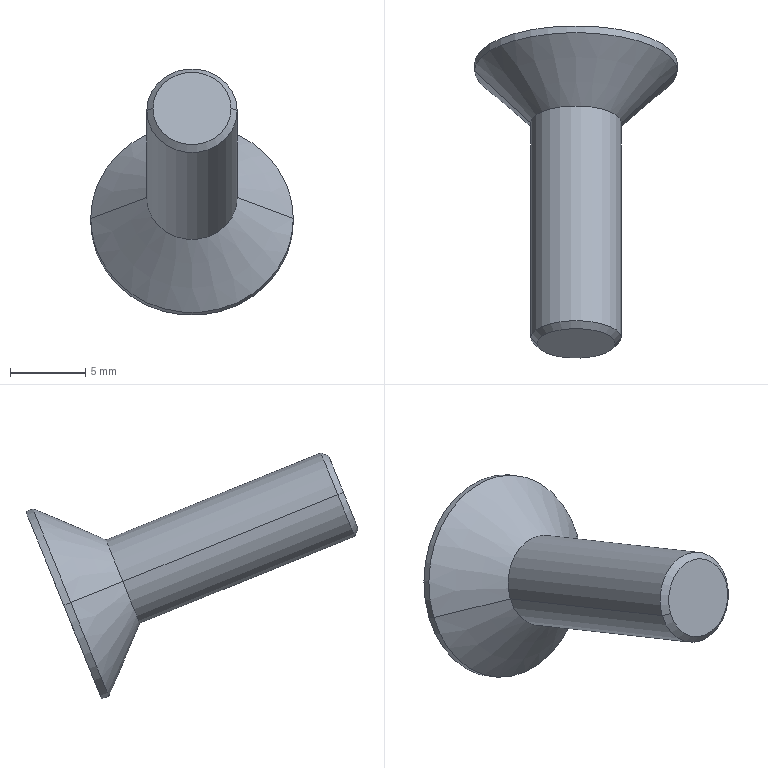Part | Creo | 1 solid | 17 faces | box 13.44 x 22.033 x 16.352 mm | volume 763.564 mm3 | plane 9 | cylinder 4 | cone 4 | commonest cylinder face diameters 6 x2 13.44 x2
STEP:
#1=CARTESIAN_POINT('',(118.28,-260.205,42.411));
#2=VERTEX_POINT('',#1);
#3=CARTESIAN_POINT('',(131.72,-260.205,42.411));
#4=VERTEX_POINT('',#3);
#5=CARTESIAN_POINT('',(125.,-260.205,42.411));
#6=DIRECTION('',(0.,0.9272,-0.3746));
#7=DIRECTION('',(-1.,0.,0.));
#8=AXIS2_PLACEMENT_3D('',#5,#6,#7);
#9=CIRCLE('',#8,6.72);
#10=EDGE_CURVE('',#2,#4,#9,.T.);
#11=ORIENTED_EDGE('',*,*,#10,.F.);
#12=CARTESIAN_POINT('',(125.,-260.205,42.411));
#13=DIRECTION('',(0.,0.9272,-0.3746));
#14=DIRECTION('',(1.,0.,0.));
#15=AXIS2_PLACEMENT_3D('',#12,#13,#14);
#16=CIRCLE('',#15,6.72);
#17=EDGE_CURVE('',#4,#2,#16,.T.);
#18=ORIENTED_EDGE('',*,*,#17,.F.);
#19=EDGE_LOOP('',(#11,#18));
#20=FACE_OUTER_BOUND('',#19,.F.);
#21=CARTESIAN_POINT('',(126.,-259.557,44.017));
#22=VERTEX_POINT('',#21);
#23=CARTESIAN_POINT('',(124.,-259.557,44.017));
#24=VERTEX_POINT('',#23);
#25=CARTESIAN_POINT('',(126.,-259.557,44.017));
#26=DIRECTION('',(-1.,0.,0.));
#27=VECTOR('',#26,2.);
#28=LINE('',#25,#27);
#29=EDGE_CURVE('',#22,#24,#28,.T.);
#30=ORIENTED_EDGE('',*,*,#29,.F.);
#31=CARTESIAN_POINT('',(127.,-260.205,42.411));
#32=VERTEX_POINT('',#31);
#33=CARTESIAN_POINT('',(127.,-260.205,42.411));
#34=DIRECTION('',(-0.5,0.3244,0.803));
#35=VECTOR('',#34,2.);
#36=LINE('',#33,#35);
#37=EDGE_CURVE('',#32,#22,#36,.T.);
#38=ORIENTED_EDGE('',*,*,#37,.F.);
#39=CARTESIAN_POINT('',(126.,-260.854,40.805));
#40=VERTEX_POINT('',#39);
#41=CARTESIAN_POINT('',(126.,-260.854,40.805));
#42=DIRECTION('',(0.5,0.3244,0.803));
#43=VECTOR('',#42,2.);
#44=LINE('',#41,#43);
#45=EDGE_CURVE('',#40,#32,#44,.T.);
#46=ORIENTED_EDGE('',*,*,#45,.F.);
#47=CARTESIAN_POINT('',(124.,-260.854,40.805));
#48=VERTEX_POINT('',#47);
#49=CARTESIAN_POINT('',(124.,-260.854,40.805));
#50=DIRECTION('',(1.,0.,0.));
#51=VECTOR('',#50,2.);
#52=LINE('',#49,#51);
#53=EDGE_CURVE('',#48,#40,#52,.T.);
#54=ORIENTED_EDGE('',*,*,#53,.F.);
#55=CARTESIAN_POINT('',(123.,-260.205,42.411));
#56=VERTEX_POINT('',#55);
#57=CARTESIAN_POINT('',(123.,-260.205,42.411));
#58=DIRECTION('',(0.5,-0.3244,-0.803));
#59=VECTOR('',#58,2.);
#60=LINE('',#57,#59);
#61=EDGE_CURVE('',#56,#48,#60,.T.);
#62=ORIENTED_EDGE('',*,*,#61,.F.);
#63=CARTESIAN_POINT('',(124.,-259.557,44.017));
#64=DIRECTION('',(-0.5,-0.3244,-0.803));
#65=VECTOR('',#64,2.);
#66=LINE('',#63,#65);
#67=EDGE_CURVE('',#24,#56,#66,.T.);
#68=ORIENTED_EDGE('',*,*,#67,.F.);
#69=EDGE_LOOP('',(#30,#38,#46,#54,#62,#68));
#70=FACE_BOUND('',#69,.F.);
#71=CARTESIAN_POINT('',(125.,-260.205,42.411));
#72=DIRECTION('',(0.,0.9272,-0.3746));
#73=DIRECTION('',(-1.,0.,0.));
#74=AXIS2_PLACEMENT_3D('',#71,#72,#73);
#75=PLANE('',#74);
#76=ADVANCED_FACE('',(#20,#70),#75,.T.);
#77=ORIENTED_EDGE('',*,*,#29,.T.);
#78=CARTESIAN_POINT('',(124.,-263.265,45.515));
#79=VERTEX_POINT('',#78);
#80=CARTESIAN_POINT('',(124.,-259.557,44.017));
#81=DIRECTION('',(0.,-0.9272,0.3746));
#82=VECTOR('',#81,4.);
#83=LINE('',#80,#82);
#84=EDGE_CURVE('',#24,#79,#83,.T.);
#85=ORIENTED_EDGE('',*,*,#84,.T.);
#86=CARTESIAN_POINT('',(126.,-263.265,45.515));
#87=VERTEX_POINT('',#86);
#88=CARTESIAN_POINT('',(126.,-263.265,45.515));
#89=DIRECTION('',(-1.,0.,0.));
#90=VECTOR('',#89,2.);
#91=LINE('',#88,#90);
#92=EDGE_CURVE('',#87,#79,#91,.T.);
#93=ORIENTED_EDGE('',*,*,#92,.F.);
#94=CARTESIAN_POINT('',(126.,-259.557,44.017));
#95=DIRECTION('',(0.,-0.9272,0.3746));
#96=VECTOR('',#95,4.);
#97=LINE('',#94,#96);
#98=EDGE_CURVE('',#22,#87,#97,.T.);
#99=ORIENTED_EDGE('',*,*,#98,.F.);
#100=EDGE_LOOP('',(#77,#85,#93,#99));
#101=FACE_OUTER_BOUND('',#100,.F.);
#102=CARTESIAN_POINT('',(124.,-263.265,45.515));
#103=DIRECTION('',(0.,0.3746,0.9272));
#104=DIRECTION('',(1.,0.,0.));
#105=AXIS2_PLACEMENT_3D('',#102,#103,#104);
#106=PLANE('',#105);
#107=ADVANCED_FACE('',(#101),#106,.F.);
#108=ORIENTED_EDGE('',*,*,#67,.T.);
#109=CARTESIAN_POINT('',(123.,-263.914,43.909));
#110=VERTEX_POINT('',#109);
#111=CARTESIAN_POINT('',(123.,-260.205,42.411));
#112=DIRECTION('',(0.,-0.9272,0.3746));
#113=VECTOR('',#112,4.);
#114=LINE('',#111,#113);
#115=EDGE_CURVE('',#56,#110,#114,.T.);
#116=ORIENTED_EDGE('',*,*,#115,.T.);
#117=CARTESIAN_POINT('',(123.,-263.914,43.909));
#118=DIRECTION('',(0.5,0.3244,0.803));
#119=VECTOR('',#118,2.);
#120=LINE('',#117,#119);
#121=EDGE_CURVE('',#110,#79,#120,.T.);
#122=ORIENTED_EDGE('',*,*,#121,.T.);
#123=ORIENTED_EDGE('',*,*,#84,.F.);
#124=EDGE_LOOP('',(#108,#116,#122,#123));
#125=FACE_OUTER_BOUND('',#124,.F.);
#126=CARTESIAN_POINT('',(123.,-263.914,43.909));
#127=DIRECTION('',(-0.866,0.1873,0.4636));
#128=DIRECTION('',(0.5,0.3244,0.803));
#129=AXIS2_PLACEMENT_3D('',#126,#127,#128);
#130=PLANE('',#129);
#131=ADVANCED_FACE('',(#125),#130,.F.);
#132=ORIENTED_EDGE('',*,*,#61,.T.);
#133=CARTESIAN_POINT('',(124.,-264.563,42.303));
#134=VERTEX_POINT('',#133);
#135=CARTESIAN_POINT('',(124.,-260.854,40.805));
#136=DIRECTION('',(0.,-0.9272,0.3746));
#137=VECTOR('',#136,4.);
#138=LINE('',#135,#137);
#139=EDGE_CURVE('',#48,#134,#138,.T.);
#140=ORIENTED_EDGE('',*,*,#139,.T.);
#141=CARTESIAN_POINT('',(124.,-264.563,42.303));
#142=DIRECTION('',(-0.5,0.3244,0.803));
#143=VECTOR('',#142,2.);
#144=LINE('',#141,#143);
#145=EDGE_CURVE('',#134,#110,#144,.T.);
#146=ORIENTED_EDGE('',*,*,#145,.T.);
#147=ORIENTED_EDGE('',*,*,#115,.F.);
#148=EDGE_LOOP('',(#132,#140,#146,#147));
#149=FACE_OUTER_BOUND('',#148,.F.);
#150=CARTESIAN_POINT('',(124.,-264.563,42.303));
#151=DIRECTION('',(-0.866,-0.1873,-0.4636));
#152=DIRECTION('',(-0.5,0.3244,0.803));
#153=AXIS2_PLACEMENT_3D('',#150,#151,#152);
#154=PLANE('',#153);
#155=ADVANCED_FACE('',(#149),#154,.F.);
#156=ORIENTED_EDGE('',*,*,#53,.T.);
#157=CARTESIAN_POINT('',(126.,-264.563,42.303));
#158=VERTEX_POINT('',#157);
#159=CARTESIAN_POINT('',(126.,-260.854,40.805));
#160=DIRECTION('',(0.,-0.9272,0.3746));
#161=VECTOR('',#160,4.);
#162=LINE('',#159,#161);
#163=EDGE_CURVE('',#40,#158,#162,.T.);
#164=ORIENTED_EDGE('',*,*,#163,.T.);
#165=CARTESIAN_POINT('',(124.,-264.563,42.303));
#166=DIRECTION('',(1.,0.,0.));
#167=VECTOR('',#166,2.);
#168=LINE('',#165,#167);
#169=EDGE_CURVE('',#134,#158,#168,.T.);
#170=ORIENTED_EDGE('',*,*,#169,.F.);
#171=ORIENTED_EDGE('',*,*,#139,.F.);
#172=EDGE_LOOP('',(#156,#164,#170,#171));
#173=FACE_OUTER_BOUND('',#172,.F.);
#174=CARTESIAN_POINT('',(126.,-264.563,42.303));
#175=DIRECTION('',(0.,-0.3746,-0.9272));
#176=DIRECTION('',(0.,-0.9272,0.3746));
#177=AXIS2_PLACEMENT_3D('',#174,#175,#176);
#178=PLANE('',#177);
#179=ADVANCED_FACE('',(#173),#178,.F.);
#180=ORIENTED_EDGE('',*,*,#45,.T.);
#181=CARTESIAN_POINT('',(127.,-263.914,43.909));
#182=VERTEX_POINT('',#181);
#183=CARTESIAN_POINT('',(127.,-260.205,42.411));
#184=DIRECTION('',(0.,-0.9272,0.3746));
#185=VECTOR('',#184,4.);
#186=LINE('',#183,#185);
#187=EDGE_CURVE('',#32,#182,#186,.T.);
#188=ORIENTED_EDGE('',*,*,#187,.T.);
#189=CARTESIAN_POINT('',(127.,-263.914,43.909));
#190=DIRECTION('',(-0.5,-0.3244,-0.803));
#191=VECTOR('',#190,2.);
#192=LINE('',#189,#191);
#193=EDGE_CURVE('',#182,#158,#192,.T.);
#194=ORIENTED_EDGE('',*,*,#193,.T.);
#195=ORIENTED_EDGE('',*,*,#163,.F.);
#196=EDGE_LOOP('',(#180,#188,#194,#195));
#197=FACE_OUTER_BOUND('',#196,.F.);
#198=CARTESIAN_POINT('',(127.,-263.914,43.909));
#199=DIRECTION('',(0.866,-0.1873,-0.4636));
#200=DIRECTION('',(-0.5,-0.3244,-0.803));
#201=AXIS2_PLACEMENT_3D('',#198,#199,#200);
#202=PLANE('',#201);
#203=ADVANCED_FACE('',(#197),#202,.F.);
#204=ORIENTED_EDGE('',*,*,#37,.T.);
#205=ORIENTED_EDGE('',*,*,#98,.T.);
#206=CARTESIAN_POINT('',(126.,-263.265,45.515));
#207=DIRECTION('',(0.5,-0.3244,-0.803));
#208=VECTOR('',#207,2.);
#209=LINE('',#206,#208);
#210=EDGE_CURVE('',#87,#182,#209,.T.);
#211=ORIENTED_EDGE('',*,*,#210,.T.);
#212=ORIENTED_EDGE('',*,*,#187,.F.);
#213=EDGE_LOOP('',(#204,#205,#211,#212));
#214=FACE_OUTER_BOUND('',#213,.F.);
#215=CARTESIAN_POINT('',(126.,-263.265,45.515));
#216=DIRECTION('',(0.866,0.1873,0.4636));
#217=DIRECTION('',(0.5,-0.3244,-0.803));
#218=AXIS2_PLACEMENT_3D('',#215,#216,#217);
#219=PLANE('',#218);
#220=ADVANCED_FACE('',(#214),#219,.F.);
#221=ORIENTED_EDGE('',*,*,#92,.T.);
#222=ORIENTED_EDGE('',*,*,#121,.F.);
#223=ORIENTED_EDGE('',*,*,#145,.F.);
#224=ORIENTED_EDGE('',*,*,#169,.T.);
#225=ORIENTED_EDGE('',*,*,#193,.F.);
#226=ORIENTED_EDGE('',*,*,#210,.F.);
#227=EDGE_LOOP('',(#221,#222,#223,#224,#225,#226));
#228=FACE_OUTER_BOUND('',#227,.F.);
#229=CARTESIAN_POINT('',(126.,-263.265,45.515));
#230=DIRECTION('',(0.,0.9272,-0.3746));
#231=DIRECTION('',(0.,-0.3746,-0.9272));
#232=AXIS2_PLACEMENT_3D('',#229,#230,#231);
#233=PLANE('',#232);
#234=ADVANCED_FACE('',(#228),#233,.T.);
#235=CARTESIAN_POINT('',(131.72,-260.669,42.598));
#236=VERTEX_POINT('',#235);
#237=CARTESIAN_POINT('',(118.28,-260.669,42.598));
#238=VERTEX_POINT('',#237);
#239=CARTESIAN_POINT('',(125.,-260.669,42.598));
#240=DIRECTION('',(0.,-0.9272,0.3746));
#241=DIRECTION('',(1.,0.,0.));
#242=AXIS2_PLACEMENT_3D('',#239,#240,#241);
#243=CIRCLE('',#242,6.72);
#244=EDGE_CURVE('',#236,#238,#243,.T.);
#245=ORIENTED_EDGE('',*,*,#244,.T.);
#246=CARTESIAN_POINT('',(118.28,-260.669,42.598));
#247=DIRECTION('',(0.,0.9272,-0.3746));
#248=VECTOR('',#247,0.5);
#249=LINE('',#246,#248);
#250=EDGE_CURVE('',#238,#2,#249,.T.);
#251=ORIENTED_EDGE('',*,*,#250,.T.);
#252=ORIENTED_EDGE('',*,*,#10,.T.);
#253=CARTESIAN_POINT('',(131.72,-260.669,42.598));
#254=DIRECTION('',(0.,0.9272,-0.3746));
#255=VECTOR('',#254,0.5);
#256=LINE('',#253,#255);
#257=EDGE_CURVE('',#236,#4,#256,.T.);
#258=ORIENTED_EDGE('',*,*,#257,.F.);
#259=EDGE_LOOP('',(#245,#251,#252,#258));
#260=FACE_OUTER_BOUND('',#259,.F.);
#261=CARTESIAN_POINT('',(125.,-259.742,42.223));
#262=DIRECTION('',(0.,0.9272,-0.3746));
#263=DIRECTION('',(-1.,0.,0.));
#264=AXIS2_PLACEMENT_3D('',#261,#262,#263);
#265=CYLINDRICAL_SURFACE('',#264,6.72);
#266=ADVANCED_FACE('',(#260),#265,.T.);
#267=CARTESIAN_POINT('',(122.,-264.118,43.991));
#268=VERTEX_POINT('',#267);
#269=CARTESIAN_POINT('',(128.,-264.118,43.991));
#270=VERTEX_POINT('',#269);
#271=CARTESIAN_POINT('',(125.,-264.118,43.991));
#272=DIRECTION('',(0.,0.9272,-0.3746));
#273=DIRECTION('',(-1.,0.,0.));
#274=AXIS2_PLACEMENT_3D('',#271,#272,#273);
#275=CIRCLE('',#274,3.);
#276=EDGE_CURVE('',#268,#270,#275,.T.);
#277=ORIENTED_EDGE('',*,*,#276,.F.);
#278=CARTESIAN_POINT('',(122.,-264.118,43.991));
#279=DIRECTION('',(-0.7071,0.6556,-0.2649));
#280=VECTOR('',#279,5.261);
#281=LINE('',#278,#280);
#282=EDGE_CURVE('',#268,#238,#281,.T.);
#283=ORIENTED_EDGE('',*,*,#282,.T.);
#284=ORIENTED_EDGE('',*,*,#244,.F.);
#285=CARTESIAN_POINT('',(128.,-264.118,43.991));
#286=DIRECTION('',(0.7071,0.6556,-0.2649));
#287=VECTOR('',#286,5.261);
#288=LINE('',#285,#287);
#289=EDGE_CURVE('',#270,#236,#288,.T.);
#290=ORIENTED_EDGE('',*,*,#289,.F.);
#291=EDGE_LOOP('',(#277,#283,#284,#290));
#292=FACE_OUTER_BOUND('',#291,.F.);
#293=CARTESIAN_POINT('',(125.,-262.394,43.295));
#294=DIRECTION('',(0.,0.9272,-0.3746));
#295=DIRECTION('',(-1.,0.,0.));
#296=AXIS2_PLACEMENT_3D('',#293,#294,#295);
#297=CONICAL_SURFACE('',#296,4.86,45.);
#298=ADVANCED_FACE('',(#292),#297,.T.);
#299=CARTESIAN_POINT('',(128.,-278.373,49.751));
#300=VERTEX_POINT('',#299);
#301=CARTESIAN_POINT('',(122.,-278.373,49.751));
#302=VERTEX_POINT('',#301);
#303=CARTESIAN_POINT('',(125.,-278.373,49.751));
#304=DIRECTION('',(0.,-0.9272,0.3746));
#305=DIRECTION('',(1.,0.,0.));
#306=AXIS2_PLACEMENT_3D('',#303,#304,#305);
#307=CIRCLE('',#306,3.);
#308=EDGE_CURVE('',#300,#302,#307,.T.);
#309=ORIENTED_EDGE('',*,*,#308,.T.);
#310=CARTESIAN_POINT('',(122.,-278.373,49.751));
#311=DIRECTION('',(0.,0.9272,-0.3746));
#312=VECTOR('',#311,15.374);
#313=LINE('',#310,#312);
#314=EDGE_CURVE('',#302,#268,#313,.T.);
#315=ORIENTED_EDGE('',*,*,#314,.T.);
#316=ORIENTED_EDGE('',*,*,#276,.T.);
#317=CARTESIAN_POINT('',(128.,-278.373,49.751));
#318=DIRECTION('',(0.,0.9272,-0.3746));
#319=VECTOR('',#318,15.374);
#320=LINE('',#317,#319);
#321=EDGE_CURVE('',#300,#270,#320,.T.);
#322=ORIENTED_EDGE('',*,*,#321,.F.);
#323=EDGE_LOOP('',(#309,#315,#316,#322));
#324=FACE_OUTER_BOUND('',#323,.F.);
#325=CARTESIAN_POINT('',(125.,-259.742,42.223));
#326=DIRECTION('',(0.,0.9272,-0.3746));
#327=DIRECTION('',(-1.,0.,0.));
#328=AXIS2_PLACEMENT_3D('',#325,#326,#327);
#329=CYLINDRICAL_SURFACE('',#328,3.);
#330=ADVANCED_FACE('',(#324),#329,.T.);
#331=CARTESIAN_POINT('',(127.594,-278.749,49.903));
#332=VERTEX_POINT('',#331);
#333=CARTESIAN_POINT('',(122.406,-278.749,49.903));
#334=VERTEX_POINT('',#333);
#335=CARTESIAN_POINT('',(125.,-278.749,49.903));
#336=DIRECTION('',(0.,-0.9272,0.3746));
#337=DIRECTION('',(1.,0.,0.));
#338=AXIS2_PLACEMENT_3D('',#335,#336,#337);
#339=CIRCLE('',#338,2.594);
#340=EDGE_CURVE('',#332,#334,#339,.T.);
#341=ORIENTED_EDGE('',*,*,#340,.T.);
#342=CARTESIAN_POINT('',(122.406,-278.749,49.903));
#343=DIRECTION('',(-0.7071,0.6556,-0.2649));
#344=VECTOR('',#343,0.5741);
#345=LINE('',#342,#344);
#346=EDGE_CURVE('',#334,#302,#345,.T.);
#347=ORIENTED_EDGE('',*,*,#346,.T.);
#348=ORIENTED_EDGE('',*,*,#308,.F.);
#349=CARTESIAN_POINT('',(127.594,-278.749,49.903));
#350=DIRECTION('',(0.7071,0.6556,-0.2649));
#351=VECTOR('',#350,0.5741);
#352=LINE('',#349,#351);
#353=EDGE_CURVE('',#332,#300,#352,.T.);
#354=ORIENTED_EDGE('',*,*,#353,.F.);
#355=EDGE_LOOP('',(#341,#347,#348,#354));
#356=FACE_OUTER_BOUND('',#355,.F.);
#357=CARTESIAN_POINT('',(125.,-278.561,49.827));
#358=DIRECTION('',(0.,0.9272,-0.3746));
#359=DIRECTION('',(-1.,0.,0.));
#360=AXIS2_PLACEMENT_3D('',#357,#358,#359);
#361=CONICAL_SURFACE('',#360,2.797,45.);
#362=ADVANCED_FACE('',(#356),#361,.T.);
#363=ORIENTED_EDGE('',*,*,#340,.F.);
#364=CARTESIAN_POINT('',(125.,-278.749,49.903));
#365=DIRECTION('',(0.,-0.9272,0.3746));
#366=DIRECTION('',(-1.,0.,0.));
#367=AXIS2_PLACEMENT_3D('',#364,#365,#366);
#368=CIRCLE('',#367,2.594);
#369=EDGE_CURVE('',#334,#332,#368,.T.);
#370=ORIENTED_EDGE('',*,*,#369,.F.);
#371=EDGE_LOOP('',(#363,#370));
#372=FACE_OUTER_BOUND('',#371,.F.);
#373=CARTESIAN_POINT('',(122.,-278.749,49.903));
#374=DIRECTION('',(0.,-0.9272,0.3746));
#375=DIRECTION('',(1.,0.,0.));
#376=AXIS2_PLACEMENT_3D('',#373,#374,#375);
#377=PLANE('',#376);
#378=ADVANCED_FACE('',(#372),#377,.T.);
#379=ORIENTED_EDGE('',*,*,#369,.T.);
#380=ORIENTED_EDGE('',*,*,#353,.T.);
#381=CARTESIAN_POINT('',(125.,-278.373,49.751));
#382=DIRECTION('',(0.,-0.9272,0.3746));
#383=DIRECTION('',(-1.,0.,0.));
#384=AXIS2_PLACEMENT_3D('',#381,#382,#383);
#385=CIRCLE('',#384,3.);
#386=EDGE_CURVE('',#302,#300,#385,.T.);
#387=ORIENTED_EDGE('',*,*,#386,.F.);
#388=ORIENTED_EDGE('',*,*,#346,.F.);
#389=EDGE_LOOP('',(#379,#380,#387,#388));
#390=FACE_OUTER_BOUND('',#389,.F.);
#391=CARTESIAN_POINT('',(125.,-278.561,49.827));
#392=DIRECTION('',(0.,0.9272,-0.3746));
#393=DIRECTION('',(-1.,0.,0.));
#394=AXIS2_PLACEMENT_3D('',#391,#392,#393);
#395=CONICAL_SURFACE('',#394,2.797,45.);
#396=ADVANCED_FACE('',(#390),#395,.T.);
#397=ORIENTED_EDGE('',*,*,#386,.T.);
#398=ORIENTED_EDGE('',*,*,#321,.T.);
#399=CARTESIAN_POINT('',(125.,-264.118,43.991));
#400=DIRECTION('',(0.,0.9272,-0.3746));
#401=DIRECTION('',(1.,0.,0.));
#402=AXIS2_PLACEMENT_3D('',#399,#400,#401);
#403=CIRCLE('',#402,3.);
#404=EDGE_CURVE('',#270,#268,#403,.T.);
#405=ORIENTED_EDGE('',*,*,#404,.T.);
#406=ORIENTED_EDGE('',*,*,#314,.F.);
#407=EDGE_LOOP('',(#397,#398,#405,#406));
#408=FACE_OUTER_BOUND('',#407,.F.);
#409=CARTESIAN_POINT('',(125.,-259.742,42.223));
#410=DIRECTION('',(0.,0.9272,-0.3746));
#411=DIRECTION('',(-1.,0.,0.));
#412=AXIS2_PLACEMENT_3D('',#409,#410,#411);
#413=CYLINDRICAL_SURFACE('',#412,3.);
#414=ADVANCED_FACE('',(#408),#413,.T.);
#415=ORIENTED_EDGE('',*,*,#404,.F.);
#416=ORIENTED_EDGE('',*,*,#289,.T.);
#417=CARTESIAN_POINT('',(125.,-260.669,42.598));
#418=DIRECTION('',(0.,-0.9272,0.3746));
#419=DIRECTION('',(-1.,0.,0.));
#420=AXIS2_PLACEMENT_3D('',#417,#418,#419);
#421=CIRCLE('',#420,6.72);
#422=EDGE_CURVE('',#238,#236,#421,.T.);
#423=ORIENTED_EDGE('',*,*,#422,.F.);
#424=ORIENTED_EDGE('',*,*,#282,.F.);
#425=EDGE_LOOP('',(#415,#416,#423,#424));
#426=FACE_OUTER_BOUND('',#425,.F.);
#427=CARTESIAN_POINT('',(125.,-262.394,43.295));
#428=DIRECTION('',(0.,0.9272,-0.3746));
#429=DIRECTION('',(-1.,0.,0.));
#430=AXIS2_PLACEMENT_3D('',#427,#428,#429);
#431=CONICAL_SURFACE('',#430,4.86,45.);
#432=ADVANCED_FACE('',(#426),#431,.T.);
#433=ORIENTED_EDGE('',*,*,#422,.T.);
#434=ORIENTED_EDGE('',*,*,#257,.T.);
#435=ORIENTED_EDGE('',*,*,#17,.T.);
#436=ORIENTED_EDGE('',*,*,#250,.F.);
#437=EDGE_LOOP('',(#433,#434,#435,#436));
#438=FACE_OUTER_BOUND('',#437,.F.);
#439=CARTESIAN_POINT('',(125.,-259.742,42.223));
#440=DIRECTION('',(0.,0.9272,-0.3746));
#441=DIRECTION('',(-1.,0.,0.));
#442=AXIS2_PLACEMENT_3D('',#439,#440,#441);
#443=CYLINDRICAL_SURFACE('',#442,6.72);
#444=ADVANCED_FACE('',(#438),#443,.T.);
#445=CLOSED_SHELL('',(#76,#107,#131,#155,#179,#203,#220,#234,#266,#298,#330,#362,#378,#396,#414,#432,#444));
#446=MANIFOLD_SOLID_BREP('',#445);
#447=(LENGTH_UNIT()NAMED_UNIT(*)SI_UNIT(.MILLI.,.METRE.));
#448=UNCERTAINTY_MEASURE_WITH_UNIT(LENGTH_MEASURE(0.003056),#447,'','');
#449=(NAMED_UNIT(*)PLANE_ANGLE_UNIT()SI_UNIT($,.RADIAN.));
#450=PLANE_ANGLE_MEASURE_WITH_UNIT(PLANE_ANGLE_MEASURE(0.01745),#449);
#451=(CONVERSION_BASED_UNIT('DEGREE',#450)NAMED_UNIT(*)PLANE_ANGLE_UNIT());
#452=(NAMED_UNIT(*)SI_UNIT($,.STERADIAN.)SOLID_ANGLE_UNIT());
#453=(GEOMETRIC_REPRESENTATION_CONTEXT(3)GLOBAL_UNCERTAINTY_ASSIGNED_CONTEXT((#448))GLOBAL_UNIT_ASSIGNED_CONTEXT((#447,#451,#452))REPRESENTATION_CONTEXT('',''));
#454=ADVANCED_BREP_SHAPE_REPRESENTATION('',(#446),#453);